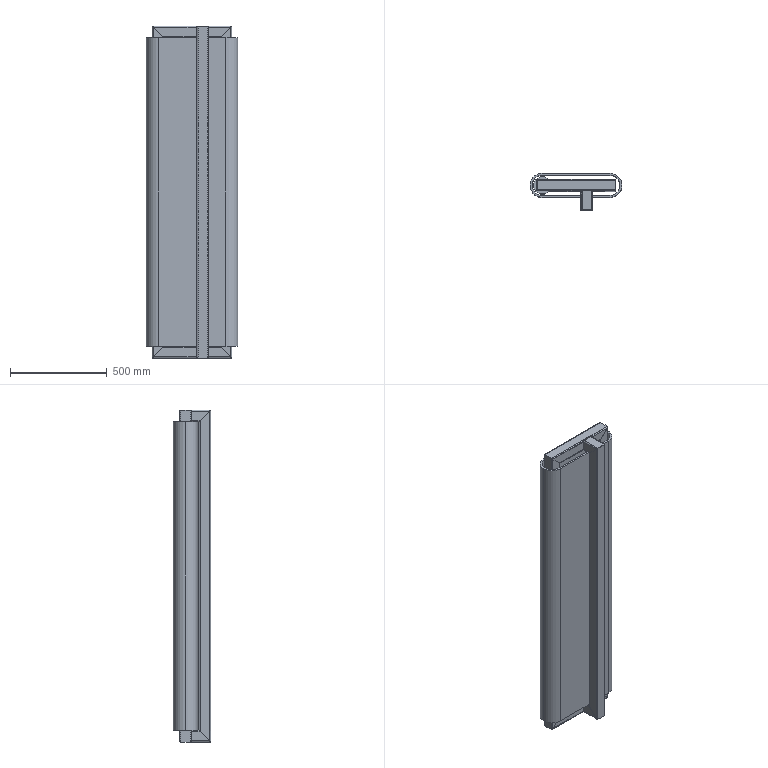Part | STEP file | Short conveyor line_Default<Machined> | 10 solids | 146 faces | box 474.996 x 192.498 x 1720 mm | volume 30115690 mm3 | plane 80 | cylinder 66 | commonest cylinder face diameters 6 x28 12 x28 104.996 x3 124.996 x3 28.065 x2 89.663 x2